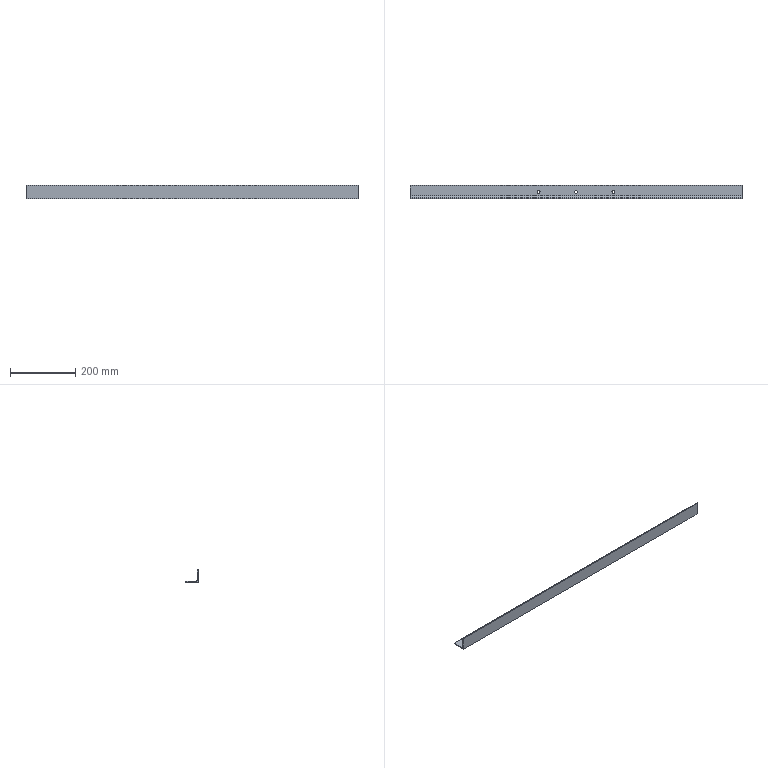Part | SolidWorks | features BaseBody 1 | 1 solid | 17 faces | box 1020 x 40 x 40 mm | volume 314011 mm3 | cylinder 9 | plane 8 | commonest cylinder face diameters 9 x6 2.667 x2 10 x1
STEP:
#1=CARTESIAN_POINT('',(399.5,20.,4.));
#2=VERTEX_POINT('',#1);
#3=CARTESIAN_POINT('',(390.5,20.,4.));
#4=VERTEX_POINT('',#3);
#5=CARTESIAN_POINT('',(395.,20.,4.));
#6=DIRECTION('',(0.,0.,-1.));
#7=DIRECTION('',(0.,1.,0.));
#8=AXIS2_PLACEMENT_3D('',#5,#6,#7);
#9=CIRCLE('',#8,4.5);
#10=EDGE_CURVE('',#2,#4,#9,.T.);
#11=ORIENTED_EDGE('',*,*,#10,.F.);
#12=CARTESIAN_POINT('',(399.5,20.,0.));
#13=VERTEX_POINT('',#12);
#14=CARTESIAN_POINT('',(399.5,20.,10.));
#15=DIRECTION('',(0.,0.,-1.));
#16=VECTOR('',#15,1000.);
#17=LINE('',#14,#16);
#18=EDGE_CURVE('',#2,#13,#17,.T.);
#19=ORIENTED_EDGE('',*,*,#18,.T.);
#20=CARTESIAN_POINT('',(390.5,20.,0.));
#21=VERTEX_POINT('',#20);
#22=CARTESIAN_POINT('',(395.,20.,0.));
#23=DIRECTION('',(0.,0.,-1.));
#24=DIRECTION('',(-1.,0.,0.));
#25=AXIS2_PLACEMENT_3D('',#22,#23,#24);
#26=CIRCLE('',#25,4.5);
#27=EDGE_CURVE('',#13,#21,#26,.T.);
#28=ORIENTED_EDGE('',*,*,#27,.T.);
#29=CARTESIAN_POINT('',(390.5,20.,10.));
#30=DIRECTION('',(0.,0.,-1.));
#31=VECTOR('',#30,1000.);
#32=LINE('',#29,#31);
#33=EDGE_CURVE('',#4,#21,#32,.T.);
#34=ORIENTED_EDGE('',*,*,#33,.F.);
#35=EDGE_LOOP('',(#11,#19,#28,#34));
#36=FACE_OUTER_BOUND('',#35,.T.);
#37=CARTESIAN_POINT('',(395.,20.,10.));
#38=DIRECTION('',(0.,0.,-1.));
#39=DIRECTION('',(-1.,0.,0.));
#40=AXIS2_PLACEMENT_3D('',#37,#38,#39);
#41=CYLINDRICAL_SURFACE('',#40,4.5);
#42=ADVANCED_FACE('',(#36),#41,.F.);
#43=CARTESIAN_POINT('',(514.5,20.,4.));
#44=VERTEX_POINT('',#43);
#45=CARTESIAN_POINT('',(505.5,20.,4.));
#46=VERTEX_POINT('',#45);
#47=CARTESIAN_POINT('',(510.,20.,4.));
#48=DIRECTION('',(0.,0.,-1.));
#49=DIRECTION('',(0.,1.,0.));
#50=AXIS2_PLACEMENT_3D('',#47,#48,#49);
#51=CIRCLE('',#50,4.5);
#52=EDGE_CURVE('',#44,#46,#51,.T.);
#53=ORIENTED_EDGE('',*,*,#52,.F.);
#54=CARTESIAN_POINT('',(514.5,20.,0.));
#55=VERTEX_POINT('',#54);
#56=CARTESIAN_POINT('',(514.5,20.,10.));
#57=DIRECTION('',(0.,0.,-1.));
#58=VECTOR('',#57,1000.);
#59=LINE('',#56,#58);
#60=EDGE_CURVE('',#44,#55,#59,.T.);
#61=ORIENTED_EDGE('',*,*,#60,.T.);
#62=CARTESIAN_POINT('',(505.5,20.,0.));
#63=VERTEX_POINT('',#62);
#64=CARTESIAN_POINT('',(510.,20.,0.));
#65=DIRECTION('',(0.,0.,-1.));
#66=DIRECTION('',(-1.,0.,0.));
#67=AXIS2_PLACEMENT_3D('',#64,#65,#66);
#68=CIRCLE('',#67,4.5);
#69=EDGE_CURVE('',#55,#63,#68,.T.);
#70=ORIENTED_EDGE('',*,*,#69,.T.);
#71=CARTESIAN_POINT('',(505.5,20.,10.));
#72=DIRECTION('',(0.,0.,-1.));
#73=VECTOR('',#72,1000.);
#74=LINE('',#71,#73);
#75=EDGE_CURVE('',#46,#63,#74,.T.);
#76=ORIENTED_EDGE('',*,*,#75,.F.);
#77=EDGE_LOOP('',(#53,#61,#70,#76));
#78=FACE_OUTER_BOUND('',#77,.T.);
#79=CARTESIAN_POINT('',(510.,20.,10.));
#80=DIRECTION('',(0.,0.,-1.));
#81=DIRECTION('',(-1.,0.,0.));
#82=AXIS2_PLACEMENT_3D('',#79,#80,#81);
#83=CYLINDRICAL_SURFACE('',#82,4.5);
#84=ADVANCED_FACE('',(#78),#83,.F.);
#85=CARTESIAN_POINT('',(629.5,20.,4.));
#86=VERTEX_POINT('',#85);
#87=CARTESIAN_POINT('',(620.5,20.,4.));
#88=VERTEX_POINT('',#87);
#89=CARTESIAN_POINT('',(625.,20.,4.));
#90=DIRECTION('',(0.,0.,-1.));
#91=DIRECTION('',(0.,1.,0.));
#92=AXIS2_PLACEMENT_3D('',#89,#90,#91);
#93=CIRCLE('',#92,4.5);
#94=EDGE_CURVE('',#86,#88,#93,.T.);
#95=ORIENTED_EDGE('',*,*,#94,.F.);
#96=CARTESIAN_POINT('',(629.5,20.,0.));
#97=VERTEX_POINT('',#96);
#98=CARTESIAN_POINT('',(629.5,20.,10.));
#99=DIRECTION('',(0.,0.,-1.));
#100=VECTOR('',#99,1000.);
#101=LINE('',#98,#100);
#102=EDGE_CURVE('',#86,#97,#101,.T.);
#103=ORIENTED_EDGE('',*,*,#102,.T.);
#104=CARTESIAN_POINT('',(620.5,20.,0.));
#105=VERTEX_POINT('',#104);
#106=CARTESIAN_POINT('',(625.,20.,0.));
#107=DIRECTION('',(0.,0.,-1.));
#108=DIRECTION('',(-1.,0.,0.));
#109=AXIS2_PLACEMENT_3D('',#106,#107,#108);
#110=CIRCLE('',#109,4.5);
#111=EDGE_CURVE('',#97,#105,#110,.T.);
#112=ORIENTED_EDGE('',*,*,#111,.T.);
#113=CARTESIAN_POINT('',(620.5,20.,10.));
#114=DIRECTION('',(0.,0.,-1.));
#115=VECTOR('',#114,1000.);
#116=LINE('',#113,#115);
#117=EDGE_CURVE('',#88,#105,#116,.T.);
#118=ORIENTED_EDGE('',*,*,#117,.F.);
#119=EDGE_LOOP('',(#95,#103,#112,#118));
#120=FACE_OUTER_BOUND('',#119,.T.);
#121=CARTESIAN_POINT('',(625.,20.,10.));
#122=DIRECTION('',(0.,0.,-1.));
#123=DIRECTION('',(-1.,0.,0.));
#124=AXIS2_PLACEMENT_3D('',#121,#122,#123);
#125=CYLINDRICAL_SURFACE('',#124,4.5);
#126=ADVANCED_FACE('',(#120),#125,.F.);
#127=CARTESIAN_POINT('',(395.,20.,0.));
#128=DIRECTION('',(0.,0.,-1.));
#129=DIRECTION('',(-1.,0.,0.));
#130=AXIS2_PLACEMENT_3D('',#127,#128,#129);
#131=CIRCLE('',#130,4.5);
#132=EDGE_CURVE('',#21,#13,#131,.T.);
#133=ORIENTED_EDGE('',*,*,#132,.F.);
#134=ORIENTED_EDGE('',*,*,#27,.F.);
#135=EDGE_LOOP('',(#133,#134));
#136=FACE_BOUND('',#135,.T.);
#137=CARTESIAN_POINT('',(510.,20.,0.));
#138=DIRECTION('',(0.,0.,-1.));
#139=DIRECTION('',(-1.,0.,0.));
#140=AXIS2_PLACEMENT_3D('',#137,#138,#139);
#141=CIRCLE('',#140,4.5);
#142=EDGE_CURVE('',#63,#55,#141,.T.);
#143=ORIENTED_EDGE('',*,*,#142,.F.);
#144=ORIENTED_EDGE('',*,*,#69,.F.);
#145=EDGE_LOOP('',(#143,#144));
#146=FACE_BOUND('',#145,.T.);
#147=CARTESIAN_POINT('',(625.,20.,0.));
#148=DIRECTION('',(0.,0.,-1.));
#149=DIRECTION('',(-1.,0.,0.));
#150=AXIS2_PLACEMENT_3D('',#147,#148,#149);
#151=CIRCLE('',#150,4.5);
#152=EDGE_CURVE('',#105,#97,#151,.T.);
#153=ORIENTED_EDGE('',*,*,#152,.F.);
#154=ORIENTED_EDGE('',*,*,#111,.F.);
#155=EDGE_LOOP('',(#153,#154));
#156=FACE_BOUND('',#155,.T.);
#157=CARTESIAN_POINT('',(0.,0.,0.));
#158=VERTEX_POINT('',#157);
#159=CARTESIAN_POINT('',(0.,40.,0.));
#160=VERTEX_POINT('',#159);
#161=CARTESIAN_POINT('',(0.,40.,0.));
#162=DIRECTION('',(0.,1.,0.));
#163=VECTOR('',#162,1000.);
#164=LINE('',#161,#163);
#165=EDGE_CURVE('',#158,#160,#164,.T.);
#166=ORIENTED_EDGE('',*,*,#165,.T.);
#167=CARTESIAN_POINT('',(1020.,40.,0.));
#168=VERTEX_POINT('',#167);
#169=CARTESIAN_POINT('',(1020.,40.,0.));
#170=DIRECTION('',(-1.,0.,0.));
#171=VECTOR('',#170,1000.);
#172=LINE('',#169,#171);
#173=EDGE_CURVE('',#168,#160,#172,.T.);
#174=ORIENTED_EDGE('',*,*,#173,.F.);
#175=CARTESIAN_POINT('',(1020.,0.,0.));
#176=VERTEX_POINT('',#175);
#177=CARTESIAN_POINT('',(1020.,40.,0.));
#178=DIRECTION('',(0.,1.,0.));
#179=VECTOR('',#178,1000.);
#180=LINE('',#177,#179);
#181=EDGE_CURVE('',#176,#168,#180,.T.);
#182=ORIENTED_EDGE('',*,*,#181,.F.);
#183=CARTESIAN_POINT('',(1020.,0.,0.));
#184=DIRECTION('',(-1.,0.,0.));
#185=VECTOR('',#184,1000.);
#186=LINE('',#183,#185);
#187=EDGE_CURVE('',#176,#158,#186,.T.);
#188=ORIENTED_EDGE('',*,*,#187,.T.);
#189=EDGE_LOOP('',(#166,#174,#182,#188));
#190=FACE_OUTER_BOUND('',#189,.T.);
#191=CARTESIAN_POINT('',(1020.,40.,0.));
#192=DIRECTION('',(0.,0.,1.));
#193=DIRECTION('',(1.,0.,0.));
#194=AXIS2_PLACEMENT_3D('',#191,#192,#193);
#195=PLANE('',#194);
#196=ADVANCED_FACE('',(#136,#146,#156,#190),#195,.F.);
#197=CARTESIAN_POINT('',(0.,40.,2.667));
#198=VERTEX_POINT('',#197);
#199=CARTESIAN_POINT('',(0.,40.,0.));
#200=DIRECTION('',(0.,0.,1.));
#201=VECTOR('',#200,1000.);
#202=LINE('',#199,#201);
#203=EDGE_CURVE('',#160,#198,#202,.T.);
#204=ORIENTED_EDGE('',*,*,#203,.T.);
#205=CARTESIAN_POINT('',(1020.,40.,2.667));
#206=VERTEX_POINT('',#205);
#207=CARTESIAN_POINT('',(1020.,40.,2.667));
#208=DIRECTION('',(-1.,0.,0.));
#209=VECTOR('',#208,1000.);
#210=LINE('',#207,#209);
#211=EDGE_CURVE('',#206,#198,#210,.T.);
#212=ORIENTED_EDGE('',*,*,#211,.F.);
#213=CARTESIAN_POINT('',(1020.,40.,0.));
#214=DIRECTION('',(0.,0.,1.));
#215=VECTOR('',#214,1000.);
#216=LINE('',#213,#215);
#217=EDGE_CURVE('',#168,#206,#216,.T.);
#218=ORIENTED_EDGE('',*,*,#217,.F.);
#219=ORIENTED_EDGE('',*,*,#173,.T.);
#220=EDGE_LOOP('',(#204,#212,#218,#219));
#221=FACE_OUTER_BOUND('',#220,.T.);
#222=CARTESIAN_POINT('',(1020.,40.,0.));
#223=DIRECTION('',(0.,-1.,0.));
#224=DIRECTION('',(0.,0.,-1.));
#225=AXIS2_PLACEMENT_3D('',#222,#223,#224);
#226=PLANE('',#225);
#227=ADVANCED_FACE('',(#221),#226,.F.);
#228=CARTESIAN_POINT('',(0.,38.667,4.));
#229=VERTEX_POINT('',#228);
#230=CARTESIAN_POINT('',(0.,38.667,2.667));
#231=DIRECTION('',(1.,0.,0.));
#232=DIRECTION('',(0.,0.,-1.));
#233=AXIS2_PLACEMENT_3D('',#230,#231,#232);
#234=CIRCLE('',#233,1.333);
#235=EDGE_CURVE('',#198,#229,#234,.T.);
#236=ORIENTED_EDGE('',*,*,#235,.T.);
#237=CARTESIAN_POINT('',(1020.,38.667,4.));
#238=VERTEX_POINT('',#237);
#239=CARTESIAN_POINT('',(1020.,38.667,4.));
#240=DIRECTION('',(-1.,0.,0.));
#241=VECTOR('',#240,1000.);
#242=LINE('',#239,#241);
#243=EDGE_CURVE('',#238,#229,#242,.T.);
#244=ORIENTED_EDGE('',*,*,#243,.F.);
#245=CARTESIAN_POINT('',(1020.,38.667,2.667));
#246=DIRECTION('',(1.,0.,0.));
#247=DIRECTION('',(0.,0.,-1.));
#248=AXIS2_PLACEMENT_3D('',#245,#246,#247);
#249=CIRCLE('',#248,1.333);
#250=EDGE_CURVE('',#206,#238,#249,.T.);
#251=ORIENTED_EDGE('',*,*,#250,.F.);
#252=ORIENTED_EDGE('',*,*,#211,.T.);
#253=EDGE_LOOP('',(#236,#244,#251,#252));
#254=FACE_OUTER_BOUND('',#253,.T.);
#255=CARTESIAN_POINT('',(1020.,38.667,2.667));
#256=DIRECTION('',(-1.,0.,0.));
#257=DIRECTION('',(0.,0.,1.));
#258=AXIS2_PLACEMENT_3D('',#255,#256,#257);
#259=CYLINDRICAL_SURFACE('',#258,1.333);
#260=ADVANCED_FACE('',(#254),#259,.T.);
#261=CARTESIAN_POINT('',(395.,20.,4.));
#262=DIRECTION('',(0.,0.,-1.));
#263=DIRECTION('',(0.,1.,0.));
#264=AXIS2_PLACEMENT_3D('',#261,#262,#263);
#265=CIRCLE('',#264,4.5);
#266=EDGE_CURVE('',#4,#2,#265,.T.);
#267=ORIENTED_EDGE('',*,*,#266,.T.);
#268=ORIENTED_EDGE('',*,*,#10,.T.);
#269=EDGE_LOOP('',(#267,#268));
#270=FACE_BOUND('',#269,.T.);
#271=CARTESIAN_POINT('',(510.,20.,4.));
#272=DIRECTION('',(0.,0.,-1.));
#273=DIRECTION('',(0.,1.,0.));
#274=AXIS2_PLACEMENT_3D('',#271,#272,#273);
#275=CIRCLE('',#274,4.5);
#276=EDGE_CURVE('',#46,#44,#275,.T.);
#277=ORIENTED_EDGE('',*,*,#276,.T.);
#278=ORIENTED_EDGE('',*,*,#52,.T.);
#279=EDGE_LOOP('',(#277,#278));
#280=FACE_BOUND('',#279,.T.);
#281=CARTESIAN_POINT('',(625.,20.,4.));
#282=DIRECTION('',(0.,0.,-1.));
#283=DIRECTION('',(0.,1.,0.));
#284=AXIS2_PLACEMENT_3D('',#281,#282,#283);
#285=CIRCLE('',#284,4.5);
#286=EDGE_CURVE('',#88,#86,#285,.T.);
#287=ORIENTED_EDGE('',*,*,#286,.T.);
#288=ORIENTED_EDGE('',*,*,#94,.T.);
#289=EDGE_LOOP('',(#287,#288));
#290=FACE_BOUND('',#289,.T.);
#291=CARTESIAN_POINT('',(0.,9.,4.));
#292=VERTEX_POINT('',#291);
#293=CARTESIAN_POINT('',(0.,9.,4.));
#294=DIRECTION('',(0.,-1.,0.));
#295=VECTOR('',#294,1000.);
#296=LINE('',#293,#295);
#297=EDGE_CURVE('',#229,#292,#296,.T.);
#298=ORIENTED_EDGE('',*,*,#297,.T.);
#299=CARTESIAN_POINT('',(1020.,9.,4.));
#300=VERTEX_POINT('',#299);
#301=CARTESIAN_POINT('',(1020.,9.,4.));
#302=DIRECTION('',(-1.,0.,0.));
#303=VECTOR('',#302,1000.);
#304=LINE('',#301,#303);
#305=EDGE_CURVE('',#300,#292,#304,.T.);
#306=ORIENTED_EDGE('',*,*,#305,.F.);
#307=CARTESIAN_POINT('',(1020.,9.,4.));
#308=DIRECTION('',(0.,-1.,0.));
#309=VECTOR('',#308,1000.);
#310=LINE('',#307,#309);
#311=EDGE_CURVE('',#238,#300,#310,.T.);
#312=ORIENTED_EDGE('',*,*,#311,.F.);
#313=ORIENTED_EDGE('',*,*,#243,.T.);
#314=EDGE_LOOP('',(#298,#306,#312,#313));
#315=FACE_OUTER_BOUND('',#314,.T.);
#316=CARTESIAN_POINT('',(1020.,9.,4.));
#317=DIRECTION('',(0.,0.,-1.));
#318=DIRECTION('',(0.,1.,0.));
#319=AXIS2_PLACEMENT_3D('',#316,#317,#318);
#320=PLANE('',#319);
#321=ADVANCED_FACE('',(#270,#280,#290,#315),#320,.F.);
#322=CARTESIAN_POINT('',(0.,4.,9.));
#323=VERTEX_POINT('',#322);
#324=CARTESIAN_POINT('',(0.,9.,9.));
#325=DIRECTION('',(-1.,0.,0.));
#326=DIRECTION('',(0.,0.,1.));
#327=AXIS2_PLACEMENT_3D('',#324,#325,#326);
#328=CIRCLE('',#327,5.);
#329=EDGE_CURVE('',#292,#323,#328,.T.);
#330=ORIENTED_EDGE('',*,*,#329,.T.);
#331=CARTESIAN_POINT('',(1020.,4.,9.));
#332=VERTEX_POINT('',#331);
#333=CARTESIAN_POINT('',(1020.,4.,9.));
#334=DIRECTION('',(-1.,0.,0.));
#335=VECTOR('',#334,1000.);
#336=LINE('',#333,#335);
#337=EDGE_CURVE('',#332,#323,#336,.T.);
#338=ORIENTED_EDGE('',*,*,#337,.F.);
#339=CARTESIAN_POINT('',(1020.,9.,9.));
#340=DIRECTION('',(-1.,0.,0.));
#341=DIRECTION('',(0.,0.,1.));
#342=AXIS2_PLACEMENT_3D('',#339,#340,#341);
#343=CIRCLE('',#342,5.);
#344=EDGE_CURVE('',#300,#332,#343,.T.);
#345=ORIENTED_EDGE('',*,*,#344,.F.);
#346=ORIENTED_EDGE('',*,*,#305,.T.);
#347=EDGE_LOOP('',(#330,#338,#345,#346));
#348=FACE_OUTER_BOUND('',#347,.T.);
#349=CARTESIAN_POINT('',(1020.,9.,9.));
#350=DIRECTION('',(-1.,0.,0.));
#351=DIRECTION('',(0.,0.,1.));
#352=AXIS2_PLACEMENT_3D('',#349,#350,#351);
#353=CYLINDRICAL_SURFACE('',#352,5.);
#354=ADVANCED_FACE('',(#348),#353,.F.);
#355=CARTESIAN_POINT('',(0.,4.,38.667));
#356=VERTEX_POINT('',#355);
#357=CARTESIAN_POINT('',(0.,4.,38.667));
#358=DIRECTION('',(0.,0.,1.));
#359=VECTOR('',#358,1000.);
#360=LINE('',#357,#359);
#361=EDGE_CURVE('',#323,#356,#360,.T.);
#362=ORIENTED_EDGE('',*,*,#361,.T.);
#363=CARTESIAN_POINT('',(1020.,4.,38.667));
#364=VERTEX_POINT('',#363);
#365=CARTESIAN_POINT('',(1020.,4.,38.667));
#366=DIRECTION('',(-1.,0.,0.));
#367=VECTOR('',#366,1000.);
#368=LINE('',#365,#367);
#369=EDGE_CURVE('',#364,#356,#368,.T.);
#370=ORIENTED_EDGE('',*,*,#369,.F.);
#371=CARTESIAN_POINT('',(1020.,4.,38.667));
#372=DIRECTION('',(0.,0.,1.));
#373=VECTOR('',#372,1000.);
#374=LINE('',#371,#373);
#375=EDGE_CURVE('',#332,#364,#374,.T.);
#376=ORIENTED_EDGE('',*,*,#375,.F.);
#377=ORIENTED_EDGE('',*,*,#337,.T.);
#378=EDGE_LOOP('',(#362,#370,#376,#377));
#379=FACE_OUTER_BOUND('',#378,.T.);
#380=CARTESIAN_POINT('',(1020.,4.,38.667));
#381=DIRECTION('',(0.,-1.,0.));
#382=DIRECTION('',(0.,0.,-1.));
#383=AXIS2_PLACEMENT_3D('',#380,#381,#382);
#384=PLANE('',#383);
#385=ADVANCED_FACE('',(#379),#384,.F.);
#386=CARTESIAN_POINT('',(0.,2.667,40.));
#387=VERTEX_POINT('',#386);
#388=CARTESIAN_POINT('',(0.,2.667,38.667));
#389=DIRECTION('',(1.,0.,0.));
#390=DIRECTION('',(0.,0.,1.));
#391=AXIS2_PLACEMENT_3D('',#388,#389,#390);
#392=CIRCLE('',#391,1.333);
#393=EDGE_CURVE('',#356,#387,#392,.T.);
#394=ORIENTED_EDGE('',*,*,#393,.T.);
#395=CARTESIAN_POINT('',(1020.,2.667,40.));
#396=VERTEX_POINT('',#395);
#397=CARTESIAN_POINT('',(1020.,2.667,40.));
#398=DIRECTION('',(-1.,0.,0.));
#399=VECTOR('',#398,1000.);
#400=LINE('',#397,#399);
#401=EDGE_CURVE('',#396,#387,#400,.T.);
#402=ORIENTED_EDGE('',*,*,#401,.F.);
#403=CARTESIAN_POINT('',(1020.,2.667,38.667));
#404=DIRECTION('',(1.,0.,0.));
#405=DIRECTION('',(0.,0.,1.));
#406=AXIS2_PLACEMENT_3D('',#403,#404,#405);
#407=CIRCLE('',#406,1.333);
#408=EDGE_CURVE('',#364,#396,#407,.T.);
#409=ORIENTED_EDGE('',*,*,#408,.F.);
#410=ORIENTED_EDGE('',*,*,#369,.T.);
#411=EDGE_LOOP('',(#394,#402,#409,#410));
#412=FACE_OUTER_BOUND('',#411,.T.);
#413=CARTESIAN_POINT('',(1020.,2.667,38.667));
#414=DIRECTION('',(-1.,0.,0.));
#415=DIRECTION('',(0.,0.,1.));
#416=AXIS2_PLACEMENT_3D('',#413,#414,#415);
#417=CYLINDRICAL_SURFACE('',#416,1.333);
#418=ADVANCED_FACE('',(#412),#417,.T.);
#419=CARTESIAN_POINT('',(0.,0.,40.));
#420=VERTEX_POINT('',#419);
#421=CARTESIAN_POINT('',(0.,0.,40.));
#422=DIRECTION('',(0.,-1.,0.));
#423=VECTOR('',#422,1000.);
#424=LINE('',#421,#423);
#425=EDGE_CURVE('',#387,#420,#424,.T.);
#426=ORIENTED_EDGE('',*,*,#425,.T.);
#427=CARTESIAN_POINT('',(1020.,0.,40.));
#428=VERTEX_POINT('',#427);
#429=CARTESIAN_POINT('',(1020.,0.,40.));
#430=DIRECTION('',(-1.,0.,0.));
#431=VECTOR('',#430,1000.);
#432=LINE('',#429,#431);
#433=EDGE_CURVE('',#428,#420,#432,.T.);
#434=ORIENTED_EDGE('',*,*,#433,.F.);
#435=CARTESIAN_POINT('',(1020.,0.,40.));
#436=DIRECTION('',(0.,-1.,0.));
#437=VECTOR('',#436,1000.);
#438=LINE('',#435,#437);
#439=EDGE_CURVE('',#396,#428,#438,.T.);
#440=ORIENTED_EDGE('',*,*,#439,.F.);
#441=ORIENTED_EDGE('',*,*,#401,.T.);
#442=EDGE_LOOP('',(#426,#434,#440,#441));
#443=FACE_OUTER_BOUND('',#442,.T.);
#444=CARTESIAN_POINT('',(1020.,0.,40.));
#445=DIRECTION('',(0.,0.,-1.));
#446=DIRECTION('',(-1.,0.,0.));
#447=AXIS2_PLACEMENT_3D('',#444,#445,#446);
#448=PLANE('',#447);
#449=ADVANCED_FACE('',(#443),#448,.F.);
#450=CARTESIAN_POINT('',(0.,0.,0.));
#451=DIRECTION('',(0.,0.,-1.));
#452=VECTOR('',#451,1000.);
#453=LINE('',#450,#452);
#454=EDGE_CURVE('',#420,#158,#453,.T.);
#455=ORIENTED_EDGE('',*,*,#454,.T.);
#456=ORIENTED_EDGE('',*,*,#187,.F.);
#457=CARTESIAN_POINT('',(1020.,0.,0.));
#458=DIRECTION('',(0.,0.,-1.));
#459=VECTOR('',#458,1000.);
#460=LINE('',#457,#459);
#461=EDGE_CURVE('',#428,#176,#460,.T.);
#462=ORIENTED_EDGE('',*,*,#461,.F.);
#463=ORIENTED_EDGE('',*,*,#433,.T.);
#464=EDGE_LOOP('',(#455,#456,#462,#463));
#465=FACE_OUTER_BOUND('',#464,.T.);
#466=CARTESIAN_POINT('',(1020.,0.,0.));
#467=DIRECTION('',(0.,1.,0.));
#468=DIRECTION('',(0.,0.,1.));
#469=AXIS2_PLACEMENT_3D('',#466,#467,#468);
#470=PLANE('',#469);
#471=ADVANCED_FACE('',(#465),#470,.F.);
#472=ORIENTED_EDGE('',*,*,#181,.T.);
#473=ORIENTED_EDGE('',*,*,#217,.T.);
#474=ORIENTED_EDGE('',*,*,#250,.T.);
#475=ORIENTED_EDGE('',*,*,#311,.T.);
#476=ORIENTED_EDGE('',*,*,#344,.T.);
#477=ORIENTED_EDGE('',*,*,#375,.T.);
#478=ORIENTED_EDGE('',*,*,#408,.T.);
#479=ORIENTED_EDGE('',*,*,#439,.T.);
#480=ORIENTED_EDGE('',*,*,#461,.T.);
#481=EDGE_LOOP('',(#472,#473,#474,#475,#476,#477,#478,#479,#480));
#482=FACE_OUTER_BOUND('',#481,.T.);
#483=CARTESIAN_POINT('',(1020.,2.667,38.667));
#484=DIRECTION('',(-1.,0.,0.));
#485=DIRECTION('',(0.,0.,1.));
#486=AXIS2_PLACEMENT_3D('',#483,#484,#485);
#487=PLANE('',#486);
#488=ADVANCED_FACE('',(#482),#487,.F.);
#489=ORIENTED_EDGE('',*,*,#165,.F.);
#490=ORIENTED_EDGE('',*,*,#454,.F.);
#491=ORIENTED_EDGE('',*,*,#425,.F.);
#492=ORIENTED_EDGE('',*,*,#393,.F.);
#493=ORIENTED_EDGE('',*,*,#361,.F.);
#494=ORIENTED_EDGE('',*,*,#329,.F.);
#495=ORIENTED_EDGE('',*,*,#297,.F.);
#496=ORIENTED_EDGE('',*,*,#235,.F.);
#497=ORIENTED_EDGE('',*,*,#203,.F.);
#498=EDGE_LOOP('',(#489,#490,#491,#492,#493,#494,#495,#496,#497));
#499=FACE_OUTER_BOUND('',#498,.T.);
#500=CARTESIAN_POINT('',(0.,2.667,38.667));
#501=DIRECTION('',(-1.,0.,0.));
#502=DIRECTION('',(0.,0.,1.));
#503=AXIS2_PLACEMENT_3D('',#500,#501,#502);
#504=PLANE('',#503);
#505=ADVANCED_FACE('',(#499),#504,.T.);
#506=ORIENTED_EDGE('',*,*,#102,.F.);
#507=ORIENTED_EDGE('',*,*,#286,.F.);
#508=ORIENTED_EDGE('',*,*,#117,.T.);
#509=ORIENTED_EDGE('',*,*,#152,.T.);
#510=EDGE_LOOP('',(#506,#507,#508,#509));
#511=FACE_OUTER_BOUND('',#510,.T.);
#512=CARTESIAN_POINT('',(625.,20.,10.));
#513=DIRECTION('',(0.,0.,-1.));
#514=DIRECTION('',(-1.,0.,0.));
#515=AXIS2_PLACEMENT_3D('',#512,#513,#514);
#516=CYLINDRICAL_SURFACE('',#515,4.5);
#517=ADVANCED_FACE('',(#511),#516,.F.);
#518=ORIENTED_EDGE('',*,*,#60,.F.);
#519=ORIENTED_EDGE('',*,*,#276,.F.);
#520=ORIENTED_EDGE('',*,*,#75,.T.);
#521=ORIENTED_EDGE('',*,*,#142,.T.);
#522=EDGE_LOOP('',(#518,#519,#520,#521));
#523=FACE_OUTER_BOUND('',#522,.T.);
#524=CARTESIAN_POINT('',(510.,20.,10.));
#525=DIRECTION('',(0.,0.,-1.));
#526=DIRECTION('',(-1.,0.,0.));
#527=AXIS2_PLACEMENT_3D('',#524,#525,#526);
#528=CYLINDRICAL_SURFACE('',#527,4.5);
#529=ADVANCED_FACE('',(#523),#528,.F.);
#530=ORIENTED_EDGE('',*,*,#18,.F.);
#531=ORIENTED_EDGE('',*,*,#266,.F.);
#532=ORIENTED_EDGE('',*,*,#33,.T.);
#533=ORIENTED_EDGE('',*,*,#132,.T.);
#534=EDGE_LOOP('',(#530,#531,#532,#533));
#535=FACE_OUTER_BOUND('',#534,.T.);
#536=CARTESIAN_POINT('',(395.,20.,10.));
#537=DIRECTION('',(0.,0.,-1.));
#538=DIRECTION('',(-1.,0.,0.));
#539=AXIS2_PLACEMENT_3D('',#536,#537,#538);
#540=CYLINDRICAL_SURFACE('',#539,4.5);
#541=ADVANCED_FACE('',(#535),#540,.F.);
#542=CLOSED_SHELL('',(#42,#84,#126,#196,#227,#260,#321,#354,#385,#418,#449,#471,#488,#505,#517,#529,#541));
#543=MANIFOLD_SOLID_BREP('',#542);
#544=CARTESIAN_POINT('',(0.,0.,0.));
#545=DIRECTION('',(0.,0.,1.));
#546=DIRECTION('',(1.,0.,0.));
#547=AXIS2_PLACEMENT_3D('',#544,#545,#546);
#548=(LENGTH_UNIT()NAMED_UNIT(*)SI_UNIT(.MILLI.,.METRE.));
#549=UNCERTAINTY_MEASURE_WITH_UNIT(LENGTH_MEASURE(0.00001),#548,'','');
#550=(NAMED_UNIT(*)PLANE_ANGLE_UNIT()SI_UNIT($,.RADIAN.));
#551=(NAMED_UNIT(*)SI_UNIT($,.STERADIAN.)SOLID_ANGLE_UNIT());
#552=(GEOMETRIC_REPRESENTATION_CONTEXT(3)GLOBAL_UNCERTAINTY_ASSIGNED_CONTEXT((#549))GLOBAL_UNIT_ASSIGNED_CONTEXT((#548,#550,#551))REPRESENTATION_CONTEXT('',''));
#553=ADVANCED_BREP_SHAPE_REPRESENTATION('',(#543,#547),#552);